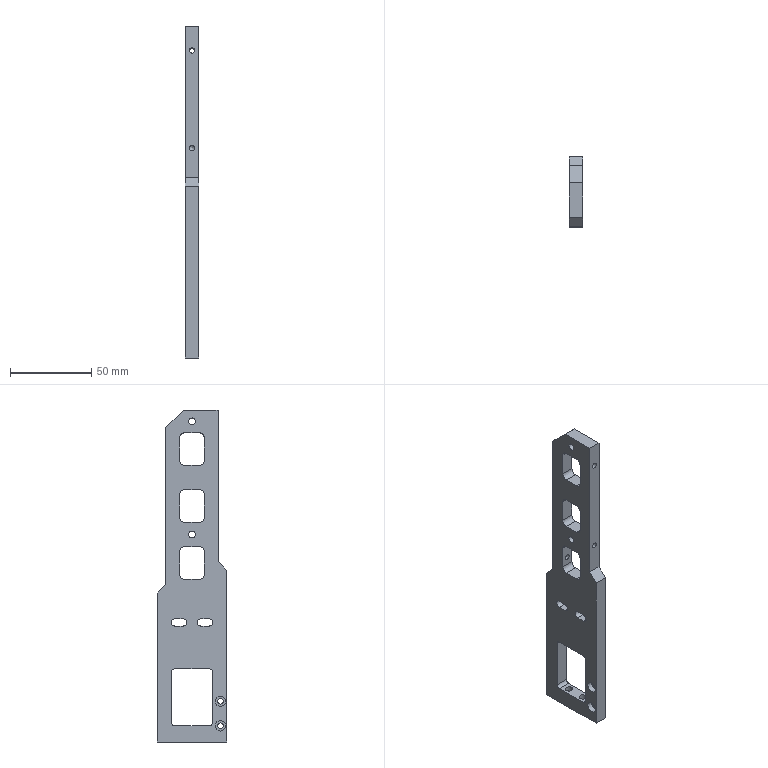Part | 1 solid | 73 faces | box 8 x 43 x 204 mm | volume 44742 mm3 | cylinder 35 | plane 33 | cone 5 | commonest cylinder face diameters 6 x13 4 x6 4.5 x6 3.3 x4 3.4 x2 4.2 x2